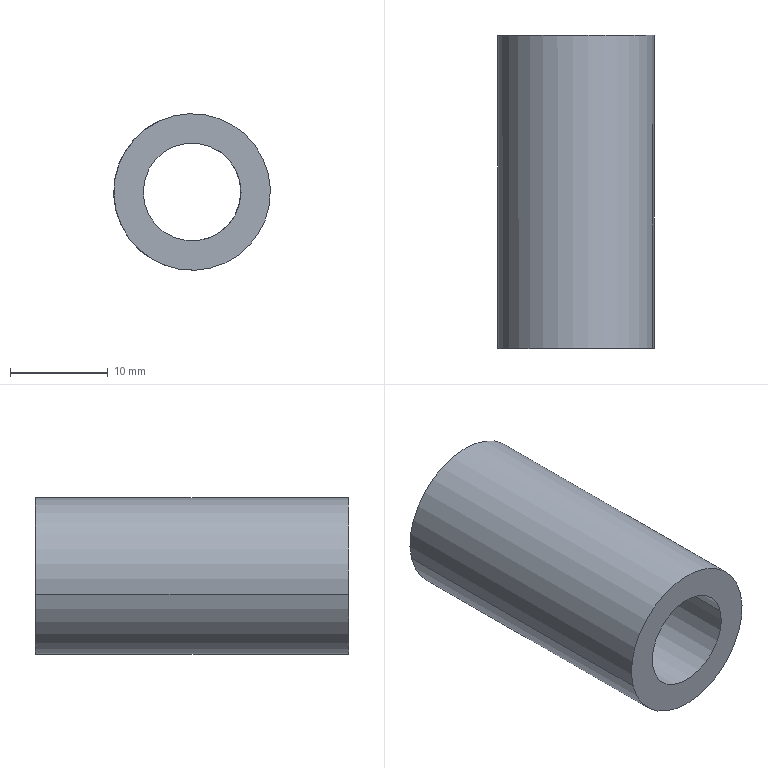Part | SolidWorks | features BaseBody 1 | 1 solid | 6 faces | box 16.031 x 32.015 x 16 mm | volume 3921 mm3 | cylinder 4 | plane 2 | commonest cylinder face diameters 10 x2 16 x2
STEP:
#1=CARTESIAN_POINT('',(337.095,390.459,105.746));
#2=VERTEX_POINT('',#1);
#3=CARTESIAN_POINT('',(346.816,390.469,108.092));
#4=VERTEX_POINT('',#3);
#5=CARTESIAN_POINT('',(341.955,390.464,106.919));
#6=DIRECTION('',(-0.0009599,1.,0.));
#7=DIRECTION('',(0.9721,0.0009331,0.2347));
#8=AXIS2_PLACEMENT_3D('',#5,#6,#7);
#9=CIRCLE('',#8,5.);
#10=EDGE_CURVE('',#2,#4,#9,.T.);
#11=ORIENTED_EDGE('',*,*,#10,.F.);
#12=CARTESIAN_POINT('',(337.064,422.459,105.746));
#13=VERTEX_POINT('',#12);
#14=CARTESIAN_POINT('',(337.095,390.459,105.746));
#15=DIRECTION('',(-0.0009599,1.,0.));
#16=VECTOR('',#15,1000.);
#17=LINE('',#14,#16);
#18=EDGE_CURVE('',#2,#13,#17,.T.);
#19=ORIENTED_EDGE('',*,*,#18,.T.);
#20=CARTESIAN_POINT('',(346.785,422.469,108.092));
#21=VERTEX_POINT('',#20);
#22=CARTESIAN_POINT('',(341.924,422.464,106.919));
#23=DIRECTION('',(0.0009599,-1.,0.));
#24=DIRECTION('',(-0.9721,-0.0009331,-0.2347));
#25=AXIS2_PLACEMENT_3D('',#22,#23,#24);
#26=CIRCLE('',#25,5.);
#27=EDGE_CURVE('',#21,#13,#26,.T.);
#28=ORIENTED_EDGE('',*,*,#27,.F.);
#29=CARTESIAN_POINT('',(346.816,390.469,108.092));
#30=DIRECTION('',(-0.0009599,1.,0.));
#31=VECTOR('',#30,1000.);
#32=LINE('',#29,#31);
#33=EDGE_CURVE('',#4,#21,#32,.T.);
#34=ORIENTED_EDGE('',*,*,#33,.F.);
#35=EDGE_LOOP('',(#11,#19,#28,#34));
#36=FACE_OUTER_BOUND('',#35,.T.);
#37=CARTESIAN_POINT('',(341.955,390.464,106.919));
#38=DIRECTION('',(-0.0009599,1.,0.));
#39=DIRECTION('',(0.9721,0.0009331,0.2347));
#40=AXIS2_PLACEMENT_3D('',#37,#38,#39);
#41=CYLINDRICAL_SURFACE('',#40,5.);
#42=ADVANCED_FACE('',(#36),#41,.F.);
#43=CARTESIAN_POINT('',(334.179,390.457,105.042));
#44=VERTEX_POINT('',#43);
#45=CARTESIAN_POINT('',(349.732,390.472,108.796));
#46=VERTEX_POINT('',#45);
#47=CARTESIAN_POINT('',(341.955,390.464,106.919));
#48=DIRECTION('',(0.0009599,-1.,0.));
#49=DIRECTION('',(0.9721,0.0009331,0.2347));
#50=AXIS2_PLACEMENT_3D('',#47,#48,#49);
#51=CIRCLE('',#50,8.);
#52=EDGE_CURVE('',#44,#46,#51,.T.);
#53=ORIENTED_EDGE('',*,*,#52,.F.);
#54=CARTESIAN_POINT('',(334.148,422.457,105.042));
#55=VERTEX_POINT('',#54);
#56=CARTESIAN_POINT('',(334.179,390.457,105.042));
#57=DIRECTION('',(-0.0009599,1.,0.));
#58=VECTOR('',#57,1000.);
#59=LINE('',#56,#58);
#60=EDGE_CURVE('',#44,#55,#59,.T.);
#61=ORIENTED_EDGE('',*,*,#60,.T.);
#62=CARTESIAN_POINT('',(349.701,422.472,108.796));
#63=VERTEX_POINT('',#62);
#64=CARTESIAN_POINT('',(341.924,422.464,106.919));
#65=DIRECTION('',(-0.0009599,1.,0.));
#66=DIRECTION('',(0.9721,0.0009331,0.2347));
#67=AXIS2_PLACEMENT_3D('',#64,#65,#66);
#68=CIRCLE('',#67,8.);
#69=EDGE_CURVE('',#63,#55,#68,.T.);
#70=ORIENTED_EDGE('',*,*,#69,.F.);
#71=CARTESIAN_POINT('',(349.732,390.472,108.796));
#72=DIRECTION('',(-0.0009599,1.,0.));
#73=VECTOR('',#72,1000.);
#74=LINE('',#71,#73);
#75=EDGE_CURVE('',#46,#63,#74,.T.);
#76=ORIENTED_EDGE('',*,*,#75,.F.);
#77=EDGE_LOOP('',(#53,#61,#70,#76));
#78=FACE_OUTER_BOUND('',#77,.T.);
#79=CARTESIAN_POINT('',(341.955,390.464,106.919));
#80=DIRECTION('',(-0.0009599,1.,0.));
#81=DIRECTION('',(0.9721,0.0009331,0.2347));
#82=AXIS2_PLACEMENT_3D('',#79,#80,#81);
#83=CYLINDRICAL_SURFACE('',#82,8.);
#84=ADVANCED_FACE('',(#78),#83,.T.);
#85=ORIENTED_EDGE('',*,*,#27,.T.);
#86=CARTESIAN_POINT('',(341.924,422.464,106.919));
#87=DIRECTION('',(0.0009599,-1.,0.));
#88=DIRECTION('',(-0.9721,-0.0009331,-0.2347));
#89=AXIS2_PLACEMENT_3D('',#86,#87,#88);
#90=CIRCLE('',#89,5.);
#91=EDGE_CURVE('',#13,#21,#90,.T.);
#92=ORIENTED_EDGE('',*,*,#91,.T.);
#93=EDGE_LOOP('',(#85,#92));
#94=FACE_BOUND('',#93,.T.);
#95=ORIENTED_EDGE('',*,*,#69,.T.);
#96=CARTESIAN_POINT('',(341.924,422.464,106.919));
#97=DIRECTION('',(-0.0009599,1.,0.));
#98=DIRECTION('',(0.9721,0.0009331,0.2347));
#99=AXIS2_PLACEMENT_3D('',#96,#97,#98);
#100=CIRCLE('',#99,8.);
#101=EDGE_CURVE('',#55,#63,#100,.T.);
#102=ORIENTED_EDGE('',*,*,#101,.T.);
#103=EDGE_LOOP('',(#95,#102));
#104=FACE_OUTER_BOUND('',#103,.T.);
#105=CARTESIAN_POINT('',(341.924,422.464,106.919));
#106=DIRECTION('',(-0.0009599,1.,0.));
#107=DIRECTION('',(0.,0.,1.));
#108=AXIS2_PLACEMENT_3D('',#105,#106,#107);
#109=PLANE('',#108);
#110=ADVANCED_FACE('',(#94,#104),#109,.T.);
#111=ORIENTED_EDGE('',*,*,#60,.F.);
#112=CARTESIAN_POINT('',(341.955,390.464,106.919));
#113=DIRECTION('',(0.0009599,-1.,0.));
#114=DIRECTION('',(0.9721,0.0009331,0.2347));
#115=AXIS2_PLACEMENT_3D('',#112,#113,#114);
#116=CIRCLE('',#115,8.);
#117=EDGE_CURVE('',#46,#44,#116,.T.);
#118=ORIENTED_EDGE('',*,*,#117,.F.);
#119=ORIENTED_EDGE('',*,*,#75,.T.);
#120=ORIENTED_EDGE('',*,*,#101,.F.);
#121=EDGE_LOOP('',(#111,#118,#119,#120));
#122=FACE_OUTER_BOUND('',#121,.T.);
#123=CARTESIAN_POINT('',(341.955,390.464,106.919));
#124=DIRECTION('',(-0.0009599,1.,0.));
#125=DIRECTION('',(0.9721,0.0009331,0.2347));
#126=AXIS2_PLACEMENT_3D('',#123,#124,#125);
#127=CYLINDRICAL_SURFACE('',#126,8.);
#128=ADVANCED_FACE('',(#122),#127,.T.);
#129=CARTESIAN_POINT('',(341.955,390.464,106.919));
#130=DIRECTION('',(-0.0009599,1.,0.));
#131=DIRECTION('',(0.9721,0.0009331,0.2347));
#132=AXIS2_PLACEMENT_3D('',#129,#130,#131);
#133=CIRCLE('',#132,5.);
#134=EDGE_CURVE('',#4,#2,#133,.T.);
#135=ORIENTED_EDGE('',*,*,#134,.T.);
#136=ORIENTED_EDGE('',*,*,#10,.T.);
#137=EDGE_LOOP('',(#135,#136));
#138=FACE_BOUND('',#137,.T.);
#139=ORIENTED_EDGE('',*,*,#117,.T.);
#140=ORIENTED_EDGE('',*,*,#52,.T.);
#141=EDGE_LOOP('',(#139,#140));
#142=FACE_OUTER_BOUND('',#141,.T.);
#143=CARTESIAN_POINT('',(341.955,390.464,106.919));
#144=DIRECTION('',(-0.0009599,1.,0.));
#145=DIRECTION('',(0.,0.,1.));
#146=AXIS2_PLACEMENT_3D('',#143,#144,#145);
#147=PLANE('',#146);
#148=ADVANCED_FACE('',(#138,#142),#147,.F.);
#149=ORIENTED_EDGE('',*,*,#18,.F.);
#150=ORIENTED_EDGE('',*,*,#134,.F.);
#151=ORIENTED_EDGE('',*,*,#33,.T.);
#152=ORIENTED_EDGE('',*,*,#91,.F.);
#153=EDGE_LOOP('',(#149,#150,#151,#152));
#154=FACE_OUTER_BOUND('',#153,.T.);
#155=CARTESIAN_POINT('',(341.955,390.464,106.919));
#156=DIRECTION('',(-0.0009599,1.,0.));
#157=DIRECTION('',(0.9721,0.0009331,0.2347));
#158=AXIS2_PLACEMENT_3D('',#155,#156,#157);
#159=CYLINDRICAL_SURFACE('',#158,5.);
#160=ADVANCED_FACE('',(#154),#159,.F.);
#161=CLOSED_SHELL('',(#42,#84,#110,#128,#148,#160));
#162=MANIFOLD_SOLID_BREP('',#161);
#163=CARTESIAN_POINT('',(0.,0.,0.));
#164=DIRECTION('',(0.,0.,1.));
#165=DIRECTION('',(1.,0.,0.));
#166=AXIS2_PLACEMENT_3D('',#163,#164,#165);
#167=(LENGTH_UNIT()NAMED_UNIT(*)SI_UNIT(.MILLI.,.METRE.));
#168=UNCERTAINTY_MEASURE_WITH_UNIT(LENGTH_MEASURE(0.00001),#167,'','');
#169=(NAMED_UNIT(*)PLANE_ANGLE_UNIT()SI_UNIT($,.RADIAN.));
#170=(NAMED_UNIT(*)SI_UNIT($,.STERADIAN.)SOLID_ANGLE_UNIT());
#171=(GEOMETRIC_REPRESENTATION_CONTEXT(3)GLOBAL_UNCERTAINTY_ASSIGNED_CONTEXT((#168))GLOBAL_UNIT_ASSIGNED_CONTEXT((#167,#169,#170))REPRESENTATION_CONTEXT('',''));
#172=ADVANCED_BREP_SHAPE_REPRESENTATION('',(#162,#166),#171);